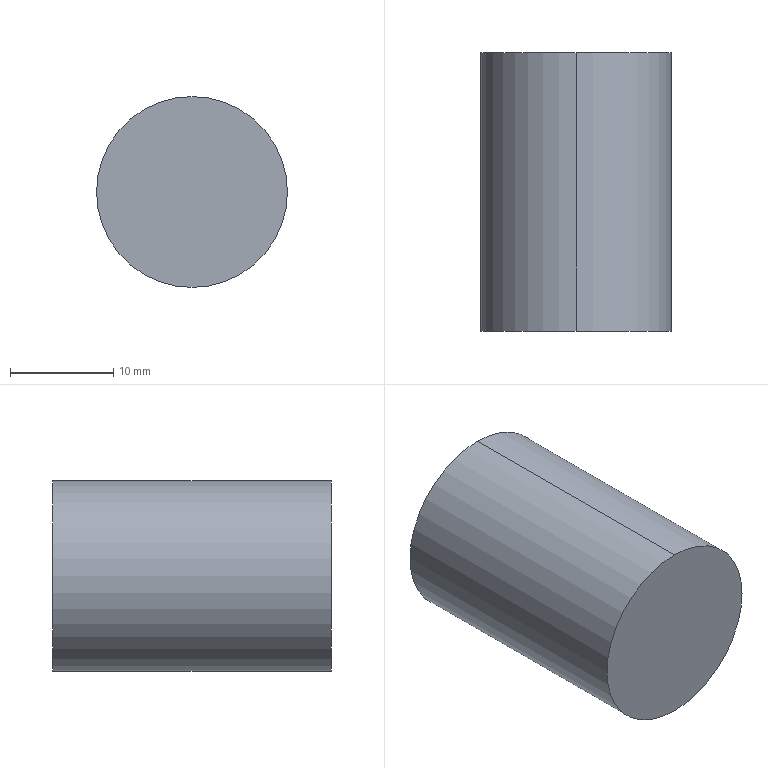Part | SolidWorks | features BaseBody 1 | 1 solid | 4 faces | box 18.5 x 27 x 18.5 mm | volume 7258 mm3 | plane 2 | cylinder 2 | commonest cylinder face diameters 18.5 x2
STEP:
#1=CARTESIAN_POINT('',(0.,27.,-9.25));
#2=VERTEX_POINT('',#1);
#3=CARTESIAN_POINT('',(0.,27.,9.25));
#4=VERTEX_POINT('',#3);
#5=CARTESIAN_POINT('',(0.,27.,0.));
#6=DIRECTION('',(0.,-1.,0.));
#7=DIRECTION('',(0.,0.,-1.));
#8=AXIS2_PLACEMENT_3D('',#5,#6,#7);
#9=CIRCLE('',#8,9.25);
#10=EDGE_CURVE('',#2,#4,#9,.T.);
#11=ORIENTED_EDGE('',*,*,#10,.F.);
#12=CARTESIAN_POINT('',(0.,27.,0.));
#13=DIRECTION('',(0.,-1.,0.));
#14=DIRECTION('',(0.,0.,-1.));
#15=AXIS2_PLACEMENT_3D('',#12,#13,#14);
#16=CIRCLE('',#15,9.25);
#17=EDGE_CURVE('',#4,#2,#16,.T.);
#18=ORIENTED_EDGE('',*,*,#17,.F.);
#19=EDGE_LOOP('',(#11,#18));
#20=FACE_OUTER_BOUND('',#19,.T.);
#21=CARTESIAN_POINT('',(0.,27.,0.));
#22=DIRECTION('',(0.,1.,0.));
#23=DIRECTION('',(1.,0.,0.));
#24=AXIS2_PLACEMENT_3D('',#21,#22,#23);
#25=PLANE('',#24);
#26=ADVANCED_FACE('',(#20),#25,.T.);
#27=CARTESIAN_POINT('',(0.,0.,-9.25));
#28=VERTEX_POINT('',#27);
#29=CARTESIAN_POINT('',(0.,0.,9.25));
#30=VERTEX_POINT('',#29);
#31=CARTESIAN_POINT('',(0.,0.,0.));
#32=DIRECTION('',(0.,1.,0.));
#33=DIRECTION('',(0.,0.,-1.));
#34=AXIS2_PLACEMENT_3D('',#31,#32,#33);
#35=CIRCLE('',#34,9.25);
#36=EDGE_CURVE('',#28,#30,#35,.T.);
#37=ORIENTED_EDGE('',*,*,#36,.F.);
#38=CARTESIAN_POINT('',(0.,0.,0.));
#39=DIRECTION('',(0.,1.,0.));
#40=DIRECTION('',(0.,0.,-1.));
#41=AXIS2_PLACEMENT_3D('',#38,#39,#40);
#42=CIRCLE('',#41,9.25);
#43=EDGE_CURVE('',#30,#28,#42,.T.);
#44=ORIENTED_EDGE('',*,*,#43,.F.);
#45=EDGE_LOOP('',(#37,#44));
#46=FACE_OUTER_BOUND('',#45,.T.);
#47=CARTESIAN_POINT('',(0.,0.,0.));
#48=DIRECTION('',(0.,1.,0.));
#49=DIRECTION('',(1.,0.,0.));
#50=AXIS2_PLACEMENT_3D('',#47,#48,#49);
#51=PLANE('',#50);
#52=ADVANCED_FACE('',(#46),#51,.F.);
#53=CARTESIAN_POINT('',(0.,15.,9.25));
#54=DIRECTION('',(0.,-1.,0.));
#55=VECTOR('',#54,1000.);
#56=LINE('',#53,#55);
#57=EDGE_CURVE('',#4,#30,#56,.T.);
#58=ORIENTED_EDGE('',*,*,#57,.F.);
#59=ORIENTED_EDGE('',*,*,#17,.T.);
#60=CARTESIAN_POINT('',(0.,15.,-9.25));
#61=DIRECTION('',(0.,-1.,0.));
#62=VECTOR('',#61,1000.);
#63=LINE('',#60,#62);
#64=EDGE_CURVE('',#2,#28,#63,.T.);
#65=ORIENTED_EDGE('',*,*,#64,.T.);
#66=ORIENTED_EDGE('',*,*,#36,.T.);
#67=EDGE_LOOP('',(#58,#59,#65,#66));
#68=FACE_OUTER_BOUND('',#67,.T.);
#69=CARTESIAN_POINT('',(0.,15.,0.));
#70=DIRECTION('',(0.,-1.,0.));
#71=DIRECTION('',(0.,0.,-1.));
#72=AXIS2_PLACEMENT_3D('',#69,#70,#71);
#73=CYLINDRICAL_SURFACE('',#72,9.25);
#74=ADVANCED_FACE('',(#68),#73,.T.);
#75=ORIENTED_EDGE('',*,*,#10,.T.);
#76=ORIENTED_EDGE('',*,*,#57,.T.);
#77=ORIENTED_EDGE('',*,*,#43,.T.);
#78=ORIENTED_EDGE('',*,*,#64,.F.);
#79=EDGE_LOOP('',(#75,#76,#77,#78));
#80=FACE_OUTER_BOUND('',#79,.T.);
#81=CARTESIAN_POINT('',(0.,15.,0.));
#82=DIRECTION('',(0.,-1.,0.));
#83=DIRECTION('',(0.,0.,-1.));
#84=AXIS2_PLACEMENT_3D('',#81,#82,#83);
#85=CYLINDRICAL_SURFACE('',#84,9.25);
#86=ADVANCED_FACE('',(#80),#85,.T.);
#87=CLOSED_SHELL('',(#26,#52,#74,#86));
#88=MANIFOLD_SOLID_BREP('',#87);
#89=CARTESIAN_POINT('',(0.,0.,0.));
#90=DIRECTION('',(0.,0.,1.));
#91=DIRECTION('',(1.,0.,0.));
#92=AXIS2_PLACEMENT_3D('',#89,#90,#91);
#93=(LENGTH_UNIT()NAMED_UNIT(*)SI_UNIT(.MILLI.,.METRE.));
#94=UNCERTAINTY_MEASURE_WITH_UNIT(LENGTH_MEASURE(0.00001),#93,'','');
#95=(NAMED_UNIT(*)PLANE_ANGLE_UNIT()SI_UNIT($,.RADIAN.));
#96=(NAMED_UNIT(*)SI_UNIT($,.STERADIAN.)SOLID_ANGLE_UNIT());
#97=(GEOMETRIC_REPRESENTATION_CONTEXT(3)GLOBAL_UNCERTAINTY_ASSIGNED_CONTEXT((#94))GLOBAL_UNIT_ASSIGNED_CONTEXT((#93,#95,#96))REPRESENTATION_CONTEXT('',''));
#98=ADVANCED_BREP_SHAPE_REPRESENTATION('',(#88,#92),#97);